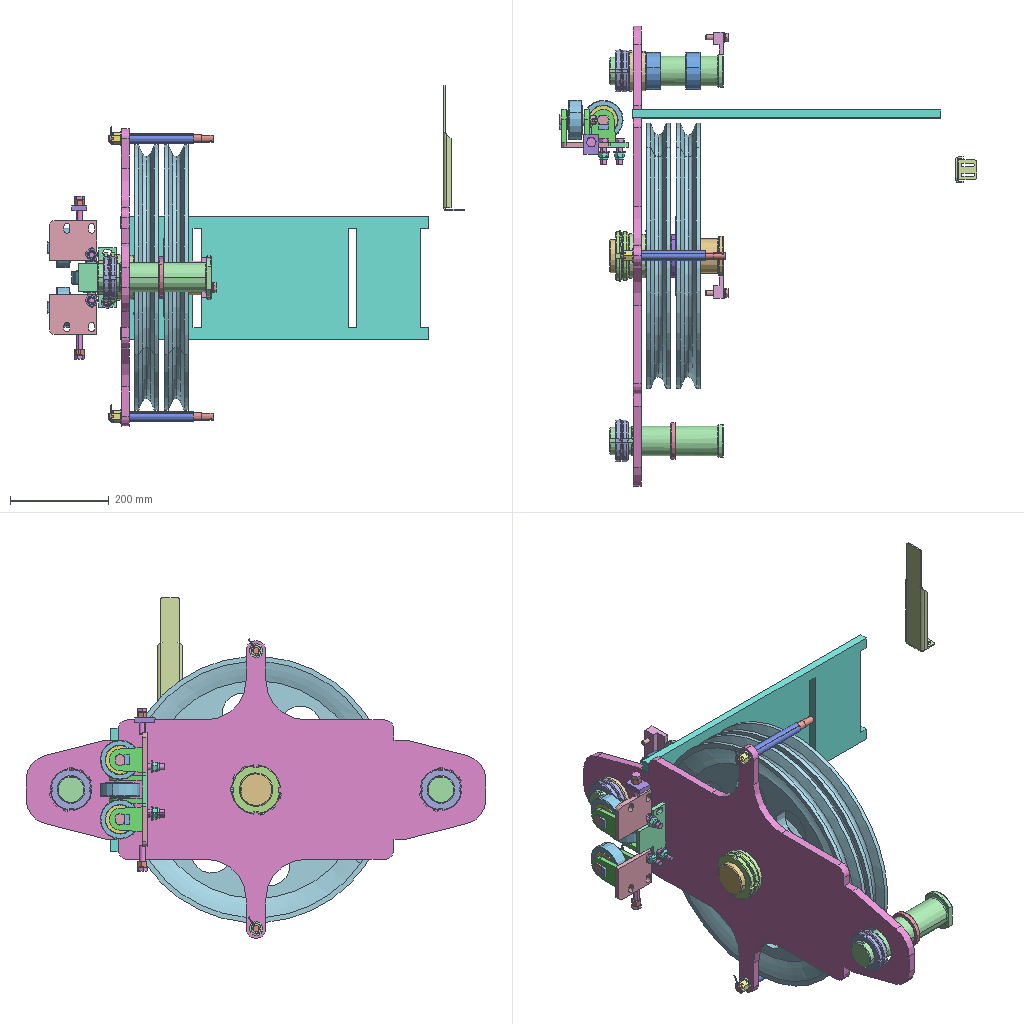Assembly | SolidWorks | 52 different items | 111 placed | box 845 x 930 x 689 mm
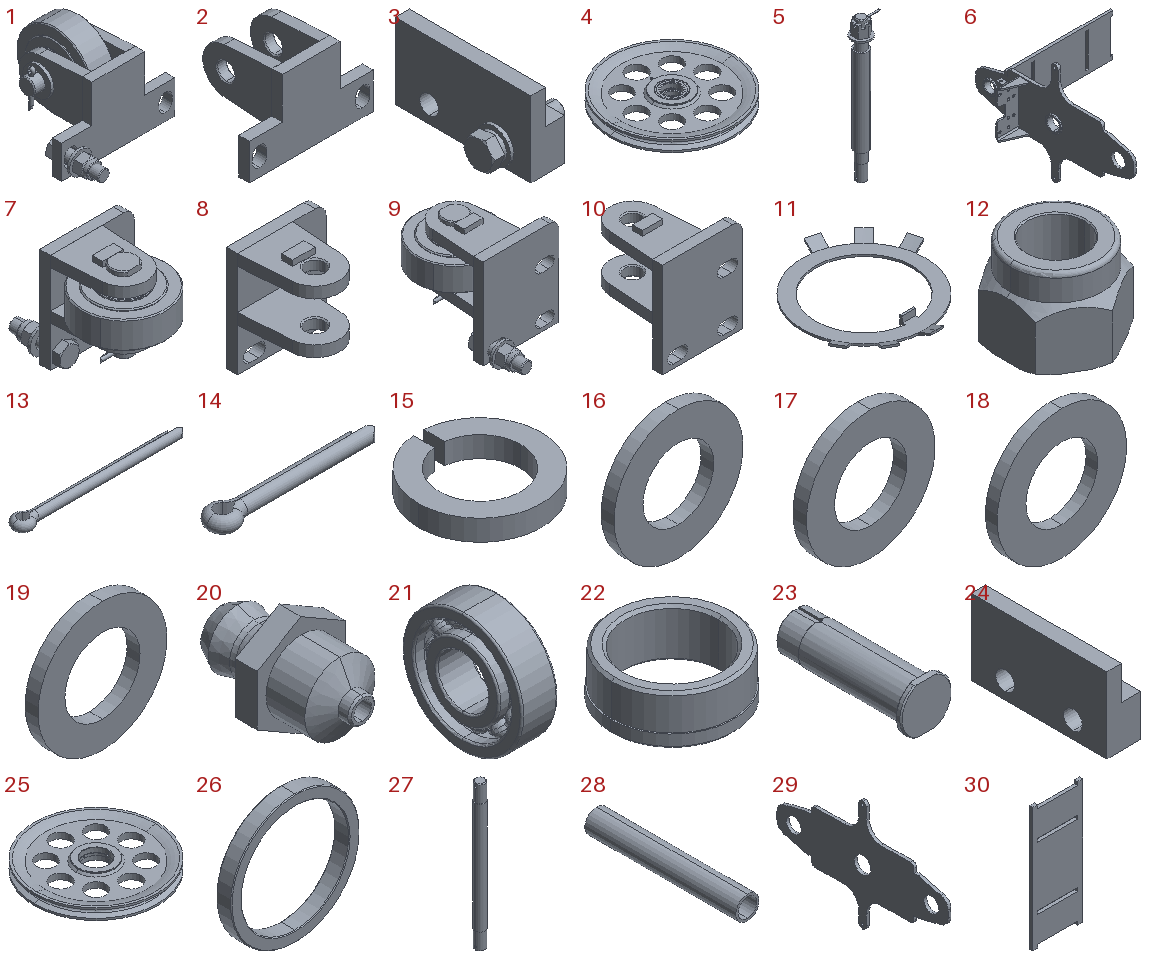Parts list (item | name | quantity | parent item | size | volume | features):
1 | (subassembly) | x1 | - | 122 x 130 x 90 mm | 267723 mm3 | features CompositeCurve 1
2 | (subassembly) | x1 | in 1 | 120 x 77 x 75 mm | 113819 mm3 | features MirrorCompFeat 1, ReferencePattern 1
3 | (subassembly) | x2 | - | 46.4 x 80 x 44.5 mm | 54258 mm3 | -
4 | (subassembly) | x2 | - | 538 x 538 x 50.446 mm | 5101431 mm3 | -
5 | (subassembly) | x2 | - | 41.5 x 28 x 212 mm | 55536 mm3 | features CompositeCurve 1
6 | (subassembly) | x1 | - | 747 x 930 x 602 mm | 6238735 mm3 | -
7 | (subassembly) | x1 | - | 95 x 130 x 102 mm | 277314 mm3 | features CompositeCurve 1
8 | (subassembly) | x1 | in 7 | 80 x 77 x 100 mm | 123411 mm3 | features LocalLPattern 1, ReferencePattern 1
9 | (subassembly) | x1 | - | 95 x 130 x 102 mm | 277314 mm3 | features CompositeCurve 1
10 | (subassembly) | x1 | in 9 | 80 x 77 x 100 mm | 123411 mm3 | features LocalLPattern 1, ReferencePattern 1
11 | - | x1 | - | 99.417 x 104.021 x 6 mm | 4358 mm3 | features Boss 1, Cut 1, Revolution 1
12 | - | x3 | in 1, 7, 9 | 17.346 x 20.03 x 14.9 mm | 2399 mm3 | features Cut 2, Chamfer 1, Extrusion 1, Revolution 1
13 | - | x2 | in 5 | 39.5 x 4.6 x 2.3 mm | 158.041 mm3 | features ICE 1, Sweep 1
14 | - | x3 | in 1, 7, 9 | 40 x 7.4 x 3.7 mm | 409.416 mm3 | features ICE 1, Sweep 1
15 | - | x2 | in 3 | 15.372 x 15.344 x 2.6 mm | 261.313 mm3 | features Extrusion 1
16 | - | x2 | in 3 | 20 x 2 x 20 mm | 438.252 mm3 | features Revolution 1
17 | - | x3 | in 1, 7, 9 | 24 x 2.5 x 24 mm | 773.126 mm3 | features Revolution 1
18 | - | x2 | in 5 | 28 x 2.5 x 28 mm | 1068 mm3 | features Revolution 1
19 | - | x3 | in 1, 7, 9 | 30 x 3 x 30 mm | 1399 mm3 | features Revolution 1
20 | - | x2 | in 4 | 10 x 16 x 11.547 mm | 627.343 mm3 | features Boss 1, Chamfer 1, Revolution 1
21 | - | x6 | in 1, 7, 9 | 12 x 40 x 40 mm | 9097 mm3 | features Revolution 5, CirPattern 2, RefAxis 1, RevCut 1
22 | - | x1 | in 6 | 92 x 92 x 36 mm | 91314 mm3 | features Chamfer 1, Revolution 1
23 | - | x1 | - | 90 x 230 x 80 mm | 896064 mm3 | features Fillet 3, ICE 2, Chamfer 1, Revolution 1
24 | - | x2 | in 3 | 20 x 80 x 44.5 mm | 48999 mm3 | features Extrusion 1, ICE 1
25 | - | x2 | in 4 | 538 x 538 x 50 mm | 4931850 mm3 | features ICE 3, Revolution 2, Chamfer 1, CirPattern 1, CombineBodies 1
26 | - | x1 | - | 85 x 10 x 85 mm | 17031 mm3 | features Chamfer 1, Extrusion 1
27 | - | x2 | in 5 | 15 x 15 x 212 mm | 36086 mm3 | features Chamfer 1, ICE 1, Revolution 1
28 | - | x2 | in 5 | 20 x 130 x 20 mm | 14703 mm3 | features Extrusion 1
29 | - | x1 | in 6 | 16 x 930 x 602 mm | 3486837 mm3 | features Extrusion 1, Fillet 1, HoleWzd 1, ICE 1
30 | - | x1 | in 6 | 250 x 16 x 623 mm | 2273312 mm3 | features Extrusion 1
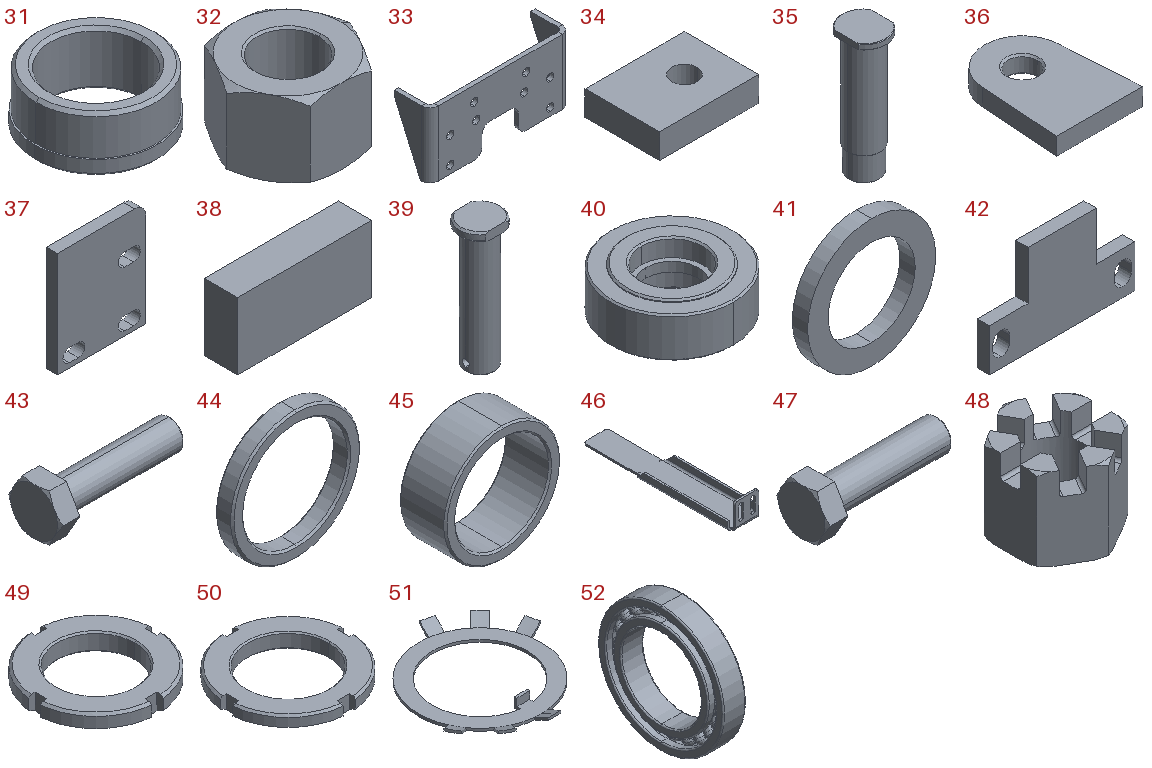31 | - | x1 | in 6 | 82 x 82 x 36 mm | 79941 mm3 | features Chamfer 1, Revolution 1
32 | - | x2 | - | 19.9 x 17.234 x 12.2 mm | 2145 mm3 | features Cut 2, Chamfer 1, Extrusion 1
33 | - | x1 | in 6 | 270 x 68.15 x 125 mm | 296148 mm3 | features Extrusion 1, FlatPattern 1, SM3dBend 1, SheetMetal 1, SolidToSheetMetal 1
34 | - | x1 | in 6 | 40 x 30 x 10 mm | 11183 mm3 | features 3DProfileFeature 1, Extrusion 1, HoleWzd 1
35 | - | x2 | - | 65 x 80 x 230 mm | 649183 mm3 | features Chamfer 2, Fillet 2, ICE 2, Revolution 1
36 | - | x6 | in 2, 8, 10 | 50 x 67 x 10 mm | 26449 mm3 | features Chamfer 1, Extrusion 1
37 | - | x2 | in 8, 10 | 80 x 10 x 95 mm | 69512 mm3 | features Extrusion 1
38 | - | x3 | in 2, 8, 10 | 20 x 5 x 10 mm | 1000 mm3 | features Extrusion 1
39 | - | x3 | in 1, 7, 9 | 24 x 20 x 75 mm | 17692 mm3 | features ICE 2, Fillet 1, Revolution 1
40 | - | x3 | in 1, 7, 9 | 80 x 80 x 29 mm | 104259 mm3 | features Chamfer 2, Revolution 2
41 | - | x6 | in 1, 7, 9 | 25 x 3 x 25 mm | 791.681 mm3 | features Extrusion 1
42 | - | x1 | in 2 | 120 x 10 x 75 mm | 59921 mm3 | features Extrusion 1
43 | - | x2 | in 3 | 46.4 x 18.475 x 16 mm | 4560 mm3 | features Chamfer 2, RevCut 2, Revolution 2, Extrusion 1, ICE 1
44 | - | x1 | - | 75 x 10 x 75 mm | 14527 mm3 | features Chamfer 1, Extrusion 1
45 | - | x2 | - | 75 x 30 x 75 mm | 44435 mm3 | features Chamfer 1, Extrusion 1
46 | - | x1 | - | 52 x 253 x 42.931 mm | 47951 mm3 | features SM3dBend 2, FlatPattern 1, SMBaseFlange 1, SheetMetal 1
47 | - | x5 | in 1, 7, 9 | 52.5 x 20.785 x 18 mm | 7195 mm3 | features Chamfer 2, RevCut 2, Revolution 2, Extrusion 1, ICE 1
48 | - | x2 | in 5 | 19.728 x 22.78 x 17.8 mm | 3522 mm3 | features Cut 3, Chamfer 1, CirPattern 1, Extrusion 1
49 | - | x4 | - | 84.623 x 84.623 x 12 mm | 36703 mm3 | features Chamfer 3, CirPattern 1, Cut 1, Extrusion 1
50 | - | x2 | - | 99.499 x 99.499 x 12 mm | 47793 mm3 | features Chamfer 3, CirPattern 1, Cut 1, Extrusion 1
51 | - | x2 | - | 85.057 x 89.139 x 6 mm | 3268 mm3 | features Boss 1, Cut 1, Revolution 1
52 | - | x4 | in 4 | 20 x 110 x 110 mm | 84477 mm3 | features Revolution 5, CirPattern 2, RefAxis 1, RevCut 1
Mates (type | each side: item.copy, entity, surface, feature):
In the top assembly
Coincident | 26.1 face plane Boss-Extrude1 | 52.1 face plane Revolve1
Coincident | 26.1 face plane Boss-Extrude1 | 52.2 face plane Revolve1
Concentric | 25.1 face cylinder CirPattern1 | 25.2 face cylinder CirPattern1
Concentric | 52.3 face cylinder Revolve1 | 23.1 face cylinder Revolve1
Concentric | 50.1 face cylinder Base-Extrude | 23.1 face cylinder Revolve1
Concentric | 50.2 face cylinder Base-Extrude | 23.1 face cylinder Revolve1
Concentric | 11.1 face cylinder Cut-Extrude2 | 23.1 face cylinder Revolve1
Coincident | assembly face | 23.1 face plane Revolve1
Concentric | assembly face | 23.1 face cylinder Revolve1
Parallel | assembly face | 23.1 face plane Cut-Extrude1
Coincident | assembly face | 52.3 face plane Revolve1
Concentric | 25.1 face cylinder Revolve1 | 25.2 face cylinder Revolve1
Parallel | 11.1 face plane Cut-Extrude2 | 50.2 face plane CirPattern1
Coincident | 11.1 face plane Base-Revolve | 50.2 face plane Base-Extrude
Coincident | 50.1 face plane Base-Extrude | 11.1 face plane Base-Revolve
Coincident | 22.1 face plane Revolve1 | 50.2 face plane Base-Extrude
Coincident | 50.1 face plane CirPattern1 | 50.2 face plane CirPattern1
Coincident | 50.1 face plane CirPattern1 | 23.1 face plane Cut-Extrude2
Concentric | assembly face | assembly face | 2 times
Concentric | assembly face | 43.1 face cylinder Revolve1
Coincident | assembly face | 24.1 face plane Boss-Extrude2
Concentric | 33.1 face cylinder Convert entities1 | assembly face | 4 times
Concentric | 33.1 face cylinder Convert entities1 | 47.1 face cylinder Revolve1
Coincident | 33.1 face plane Convert entities1 | 42.1 face plane Boss-Extrude1
Coincident | 33.1 face plane Convert entities1 | 37.1 face plane Boss-Extrude1
Parallel | 33.1 face plane Convert entities1 | 37.1 face plane Boss-Extrude1
Coincident | 37.1 face plane Boss-Extrude1 | 37.2 face plane Boss-Extrude1
Concentric | 35.1 face cylinder Revolve1 | 49.1 face cylinder Base-Extrude
Concentric | 49.2 face cylinder Base-Extrude | 35.1 face cylinder Revolve1
Concentric | 51.1 face cylinder Cut-Extrude2 | 35.1 face cylinder Revolve1
Concentric | 45.1 face cylinder Boss-Extrude1 | 35.1 face cylinder Revolve1
Concentric | 35.1 face cylinder Revolve1 | 45.2 face cylinder Boss-Extrude1
Coincident | 51.1 face plane Base-Revolve | 49.1 face plane Base-Extrude
Coincident | 49.2 face plane Base-Extrude | 51.1 face plane Base-Revolve
Concentric | assembly face | 35.1 face cylinder Revolve1
Coincident | assembly face | 35.1 face plane Revolve1
Parallel | 30.1 face plane Boss-Extrude1 | 35.1 face plane Cut-Extrude3
Coincident | assembly face | 45.1 face plane Boss-Extrude1
Coincident | 31.1 face plane Revolve1 | 45.2 face plane Boss-Extrude1
Coincident | 31.1 face plane Revolve1 | 49.2 face plane Base-Extrude
Coincident | 49.2 face plane CirPattern1 | 49.1 face plane CirPattern1
Parallel | 51.1 face plane Cut-Extrude2 | 35.1 face plane Cut-Extrude1
Parallel | 49.2 face plane CirPattern1 | 35.1 face plane Cut-Extrude1
Concentric | 49.3 face cylinder Base-Extrude | 35.2 face cylinder Revolve1
Concentric | 51.2 face cylinder Cut-Extrude2 | 35.2 face cylinder Revolve1
Concentric | 35.2 face cylinder Revolve1 | 49.4 face cylinder Base-Extrude
Coincident | 49.3 face plane CirPattern1 | 49.4 face plane CirPattern1
Parallel | 51.2 face plane Cut-Extrude2 | 35.2 face plane Cut-Extrude1
Coincident | 51.2 face plane Base-Revolve | 49.4 face plane Base-Extrude
Coincident | 49.3 face plane Base-Extrude | 51.2 face plane Base-Revolve
Parallel | 49.3 face plane CirPattern1 | 35.2 face plane Cut-Extrude1
Concentric | assembly face | 35.2 face cylinder Revolve1
Coincident | assembly face | 35.2 face plane Revolve1
Coincident | assembly face | 49.3 face plane Base-Extrude
Concentric | 44.1 face cylinder Boss-Extrude1 | 35.2 face cylinder Revolve1
DistanceDim | 44.1 face plane Boss-Extrude1 | assembly face
Parallel | 35.1 face plane Cut-Extrude3 | 24.2 face plane Boss-Extrude2
Coincident | assembly face | 24.2 face plane Boss-Extrude2
Concentric | assembly face | 28.1 face cylinder Boss-Extrude1
Coincident | assembly face | assembly edge
Concentric | assembly face | 28.2 face cylinder Boss-Extrude1
Coincident | 27.1 face plane Revolve1 | 27.2 face plane Revolve1
Concentric | 32.1 face cylinder Base-Extrude | 47.2 face cylinder Revolve1
Concentric | 34.1 face cylinder M12 Tapped Hole1 | 47.2 face cylinder Revolve1
Coincident | 34.1 face plane Boss-Extrude1 | 32.1 face plane Base-Extrude
Coincident | 32.1 face plane Base-Extrude | 47.2 face plane Boss-Extrude1
Concentric | 32.2 face cylinder Base-Extrude | 47.3 face cylinder Revolve1
Coincident | 32.2 face plane Base-Extrude | 47.3 face plane Boss-Extrude1
Concentric | assembly face | 47.3 face cylinder Revolve1
Coincident | assembly face | 32.2 face plane Base-Extrude
Coincident | assembly face | 46.1 face plane Base-Flange1
DistanceDim | 46.1 face plane Base-Flange1 | assembly face | 2 times
In subassembly 4
Coordinate | 25.3 select_type:25 | 4.1 select_type:11
Concentric | 25.3 face cylinder Revolve1 | 52.4 face cylinder Revolve1
Coincident | 25.3 face plane Revolve1 | 52.4 face plane Revolve1
Concentric | 25.3 face cylinder Revolve1 | 52.5 face cylinder Revolve1
Coincident | 25.3 face plane Revolve1 | 52.5 face plane Revolve1
Concentric | 25.3 face cylinder Combine1 | 20.1 face cylinder Revolve2
In subassembly 7
Concentric | 40.1 face cylinder Revolve2 | 39.1 face cylinder Revolve1
Concentric | 40.1 face cylinder Revolve2 | 19.1 face cylinder Base-Revolve
Concentric | 40.1 face cylinder Revolve2 | 21.1 face cylinder Revolve1
Concentric | 39.1 face cylinder Revolve1 | 21.2 face cylinder Revolve1
Concentric | 41.1 face cylinder Boss-Extrude1 | 39.1 face cylinder Revolve1
Concentric | 39.1 face cylinder Revolve1 | 41.2 face cylinder Boss-Extrude1
Concentric | 36.1 face cylinder Boss-Extrude1 | 39.1 face cylinder Revolve1
Coincident | 40.1 face plane Revolve2 | 21.2 face plane Revolve1
Coincident | 41.2 face plane Boss-Extrude1 | 21.2 face plane Revolve1
Coincident | 40.1 face plane Revolve2 | 21.1 face plane Revolve1
Coincident | 41.1 face plane Boss-Extrude1 | 21.1 face plane Revolve1
Coincident | 36.1 face plane Boss-Extrude1 | 41.2 face plane Boss-Extrude1
Parallel | 38.1 face plane Boss-Extrude1 | 39.1 face plane Cut-Extrude2
Concentric | 39.1 face cylinder Cut-Extrude1 | 14.1 face cylinder Sweep2
Parallel | 39.1 face plane Cut-Extrude2 | 14.1 face plane Sweep2
Tangent | 39.1 face cylinder Revolve1 | 14.1 edge
Concentric | 47.2 face cylinder Revolve1 | 12.1 face cylinder Base-Extrude
Concentric | 47.2 face cylinder Revolve1 | 17.1 face cylinder Base-Revolve
Coincident | 12.1 face plane Base-Extrude | 17.1 face plane Base-Revolve
Slot | 47.2 face cylinder Revolve1 | 37.3 face plane Boss-Extrude1
Coincident | 37.3 face plane Boss-Extrude1 | 47.2 face plane Boss-Extrude1
DistanceDim | 17.1 face plane Base-Revolve | 37.3 face plane Boss-Extrude1
Coincident | 36.2 face plane Boss-Extrude1 | 39.1 face plane Revolve1
Coincident | 36.1 face plane Boss-Extrude1 | 19.1 face plane Base-Revolve
In subassembly 8
Coincident | 36.3 face plane Boss-Extrude1 | 37.4 face plane Boss-Extrude1 | 2 times
Coincident | 36.3 face plane Boss-Extrude1 | 38.2 face plane Boss-Extrude1
DistanceDim | 38.2 face plane Boss-Extrude1 | 36.3 face cylinder Boss-Extrude1
DistanceDim | 37.4 face plane Boss-Extrude1 | 38.2 face plane Boss-Extrude1
Parallel | 37.4 face plane Boss-Extrude1 | 38.2 face plane Boss-Extrude1
Coincident | 36.3 edge | 37.4 face plane Boss-Extrude1
In subassembly 3
Concentric | 15.1 face cylinder Extrude1 | 43.2 face cylinder Revolve1
Concentric | 16.1 face cylinder Base-Revolve | 43.2 face cylinder Revolve1
Coincident | 15.1 face plane Extrude1 | 43.2 face plane Boss-Extrude1
Coincident | 15.1 face plane Extrude1 | 16.1 face plane Base-Revolve
Concentric | 24.3 face cylinder Boss-Extrude2 | 43.2 face cylinder Revolve1
Coincident | 24.3 face plane Boss-Extrude1 | 16.1 face plane Base-Revolve
In subassembly 1
Concentric | 40.1 face cylinder Revolve2 | 39.1 face cylinder Revolve1
Concentric | 40.1 face cylinder Revolve2 | 19.1 face cylinder Base-Revolve
Concentric | 40.1 face cylinder Revolve2 | 21.1 face cylinder Revolve1
Concentric | 39.1 face cylinder Revolve1 | 21.2 face cylinder Revolve1
Concentric | 41.1 face cylinder Boss-Extrude1 | 39.1 face cylinder Revolve1
Concentric | 39.1 face cylinder Revolve1 | 41.2 face cylinder Boss-Extrude1
Concentric | 36.4 face cylinder Boss-Extrude1 | 39.1 face cylinder Revolve1
Coincident | 40.1 face plane Revolve2 | 21.2 face plane Revolve1
Coincident | 41.2 face plane Boss-Extrude1 | 21.2 face plane Revolve1
Coincident | 40.1 face plane Revolve2 | 21.1 face plane Revolve1
Coincident | 41.1 face plane Boss-Extrude1 | 21.1 face plane Revolve1
Coincident | 36.4 face plane Boss-Extrude1 | 41.2 face plane Boss-Extrude1
Coincident | 36.5 face plane Boss-Extrude1 | 19.1 face plane Base-Revolve
Coincident | 36.4 face plane Boss-Extrude1 | 39.1 face plane Revolve1
Parallel | 38.3 face plane Boss-Extrude1 | 39.1 face plane Cut-Extrude2
Concentric | 39.1 face cylinder Cut-Extrude1 | 14.1 face cylinder Sweep2
Parallel | 39.1 face plane Cut-Extrude2 | 14.1 face plane Sweep2
Tangent | 39.1 face cylinder Revolve1 | 14.1 edge
Concentric | 47.2 face cylinder Revolve1 | 12.1 face cylinder Base-Extrude
Concentric | 47.2 face cylinder Revolve1 | 17.1 face cylinder Base-Revolve
Coincident | 12.1 face plane Base-Extrude | 17.1 face plane Base-Revolve
Slot | 47.2 face cylinder Revolve1 | 42.2 face plane Boss-Extrude1
Coincident | 42.2 face plane Boss-Extrude1 | 47.2 face plane Boss-Extrude1
DistanceDim | 17.1 face plane Base-Revolve | 42.2 face plane Boss-Extrude1
In subassembly 2
Coincident | 42.3 face plane Boss-Extrude1 | 36.3 face plane Boss-Extrude1 | 2 times
Coincident | 42.3 face plane Boss-Extrude1 | 36.3 edge
Coincident | 38.2 face plane Boss-Extrude1 | 36.6 face plane Boss-Extrude1
DistanceDim | 38.2 face plane Boss-Extrude1 | 42.3 face plane Boss-Extrude1
Width | 38.2 face plane Boss-Extrude1 | 38.2 face plane Boss-Extrude1 | 36.6 face plane Boss-Extrude1 | 36.6 face plane Boss-Extrude1
In subassembly 6
DistanceDim | 29.1 face plane Boss-Extrude1 | 6.1 plane
DistanceDim | 29.1 face cylinder Boss-Extrude1 | 6.1 plane | 2 times
Parallel | 29.1 face plane Boss-Extrude1 | 6.1 plane
Coincident | 29.1 face plane Boss-Extrude1 | 30.2 face plane Boss-Extrude1 | 3 times
Concentric | 29.1 face cylinder Boss-Extrude1 | 31.2 face cylinder Revolve1
Coincident | 29.1 face plane Boss-Extrude1 | 31.2 face plane Revolve1
Coincident | 29.1 face plane Boss-Extrude1 | 33.2 face plane Convert entities1
Parallel | 29.1 face plane Boss-Extrude1 | 33.2 face plane Convert entities1
Coincident | 33.2 edge | 6.1 plane
DistanceDim | 33.2 face plane Convert entities1 | 6.1 plane
DistanceDim | 34.2 face plane Boss-Extrude1 | 33.2 face plane Convert entities1
DistanceDim | 33.2 face plane Sketch bend2 | 34.2 face plane Boss-Extrude1
Coincident | 33.2 face plane Convert entities1 | 34.2 face plane Boss-Extrude1
Concentric | 29.1 face cylinder Boss-Extrude1 | 22.2 face cylinder Revolve1
Coincident | 29.1 face plane Boss-Extrude1 | 22.2 face plane Revolve1
In subassembly 5
Concentric | 27.3 face cylinder Revolve1 | 28.3 face cylinder Boss-Extrude1
Width | 28.3 face plane Boss-Extrude1 | 28.3 face plane Boss-Extrude1 | 27.3 face plane Revolve1 | 27.3 face plane Revolve1
Concentric | 27.3 face cylinder Revolve1 | 18.1 face cylinder Base-Revolve
Coincident | 27.3 face plane Revolve1 | 18.1 face plane Base-Revolve
Coincident | 18.1 face plane Base-Revolve | 48.1 face plane Base-Extrude
Concentric | 27.3 face cylinder Revolve1 | 48.1 face cylinder Base-Extrude
Concentric | 27.3 face cylinder Cut-Extrude1 | 13.1 face cylinder Sweep2
Parallel | 48.1 face plane Base-Extrude | 13.1 face plane Sweep2
Tangent | 27.3 face cylinder Revolve1 | 13.1 edge
In subassembly 9
Concentric | 40.1 face cylinder Revolve2 | 39.1 face cylinder Revolve1
Concentric | 40.1 face cylinder Revolve2 | 19.1 face cylinder Base-Revolve
Concentric | 40.1 face cylinder Revolve2 | 21.1 face cylinder Revolve1
Concentric | 39.1 face cylinder Revolve1 | 21.2 face cylinder Revolve1
Concentric | 41.1 face cylinder Boss-Extrude1 | 39.1 face cylinder Revolve1
Concentric | 39.1 face cylinder Revolve1 | 41.2 face cylinder Boss-Extrude1
Concentric | 36.7 face cylinder Boss-Extrude1 | 39.1 face cylinder Revolve1
Coincident | 40.1 face plane Revolve2 | 21.2 face plane Revolve1
Coincident | 41.2 face plane Boss-Extrude1 | 21.2 face plane Revolve1
Coincident | 40.1 face plane Revolve2 | 21.1 face plane Revolve1
Coincident | 41.1 face plane Boss-Extrude1 | 21.1 face plane Revolve1
Coincident | 36.7 face plane Boss-Extrude1 | 41.2 face plane Boss-Extrude1
Parallel | 38.4 face plane Boss-Extrude1 | 39.1 face plane Cut-Extrude2
Concentric | 39.1 face cylinder Cut-Extrude1 | 14.1 face cylinder Sweep2
Parallel | 39.1 face plane Cut-Extrude2 | 14.1 face plane Sweep2
Tangent | 39.1 face cylinder Revolve1 | 14.1 edge
Concentric | 47.2 face cylinder Revolve1 | 12.1 face cylinder Base-Extrude
Concentric | 47.2 face cylinder Revolve1 | 17.1 face cylinder Base-Revolve
Coincident | 12.1 face plane Base-Extrude | 17.1 face plane Base-Revolve
Slot | 47.2 face cylinder Revolve1 | 37.5 face plane Boss-Extrude1
Coincident | 37.5 face plane Boss-Extrude1 | 47.2 face plane Boss-Extrude1
DistanceDim | 17.1 face plane Base-Revolve | 37.5 face plane Boss-Extrude1
Coincident | 36.8 face plane Boss-Extrude1 | 39.1 face plane Revolve1
Coincident | 36.7 face plane Boss-Extrude1 | 19.1 face plane Base-Revolve
In subassembly 10
Coincident | 36.3 face plane Boss-Extrude1 | 37.4 face plane Boss-Extrude1 | 2 times
Coincident | 36.3 face plane Boss-Extrude1 | 38.2 face plane Boss-Extrude1
DistanceDim | 38.2 face plane Boss-Extrude1 | 36.3 face cylinder Boss-Extrude1
DistanceDim | 36.6 edge | 37.4 face plane Boss-Extrude1
DistanceDim | 37.4 face plane Boss-Extrude1 | 38.2 face plane Boss-Extrude1
Parallel | 37.4 face plane Boss-Extrude1 | 38.2 face plane Boss-Extrude1